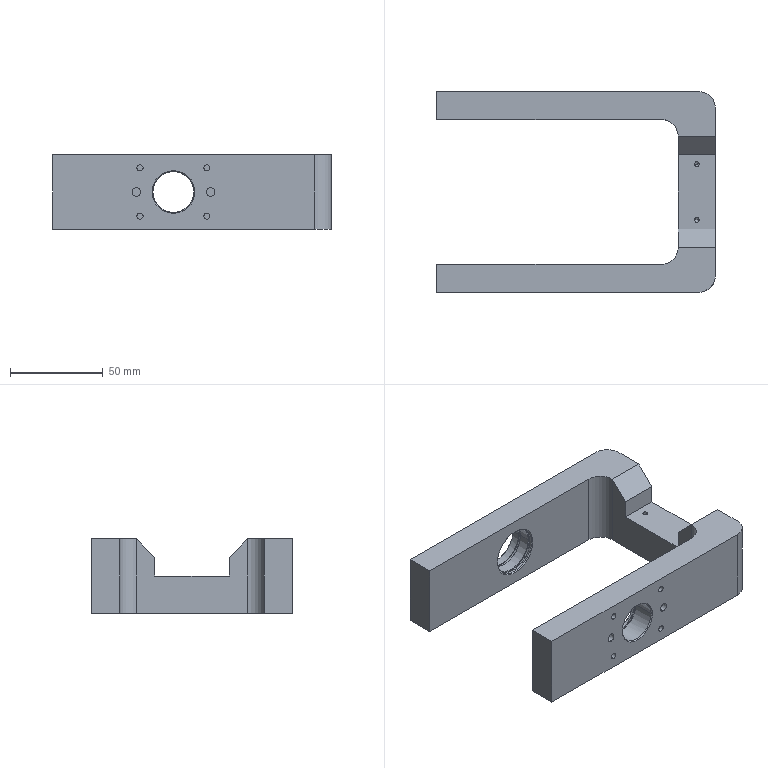Part | SolidWorks | features ICE 6, 3DProfileFeature 4, HoleWzd 4, Chamfer 1, Extrusion 1, LPattern 1 | 1 solid | 82 faces | box 150 x 108 x 40 mm | volume 209243 mm3 | cylinder 42 | plane 22 | cone 18 | commonest cylinder face diameters 3.3 x10 2.5 x8 26 x6 4.5 x4 18 x4 22 x4